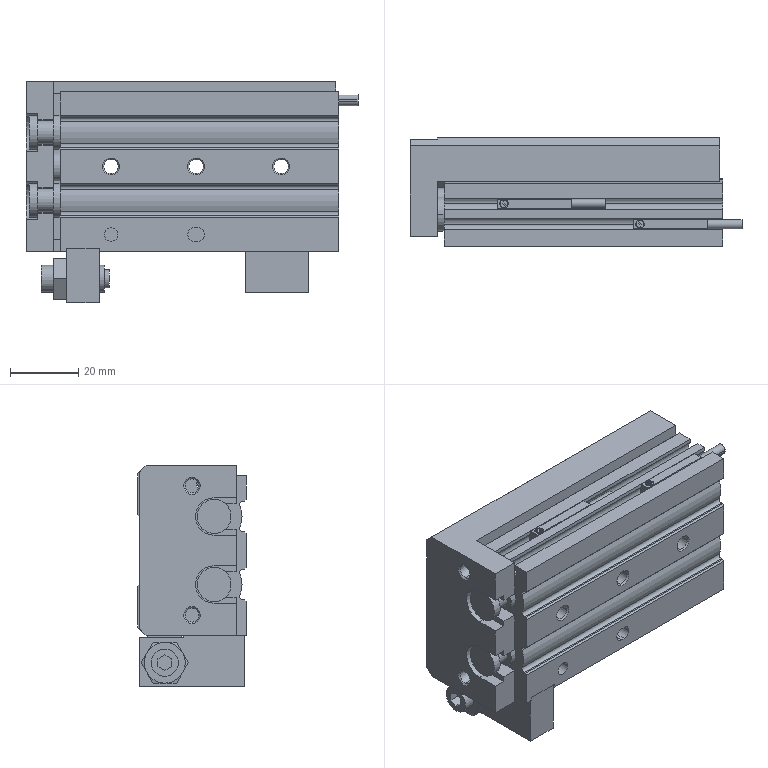Part | SolidWorks | features AEMSimFeature 1 | 8 solids | 487 faces | box 97.6 x 32 x 65 mm | volume 120798 mm3 | plane 255 | cylinder 166 | cone 66 | commonest cylinder face diameters 3.242 x24 4 x18 4.2 x10 7.5 x10 4.134 x8 6 x8